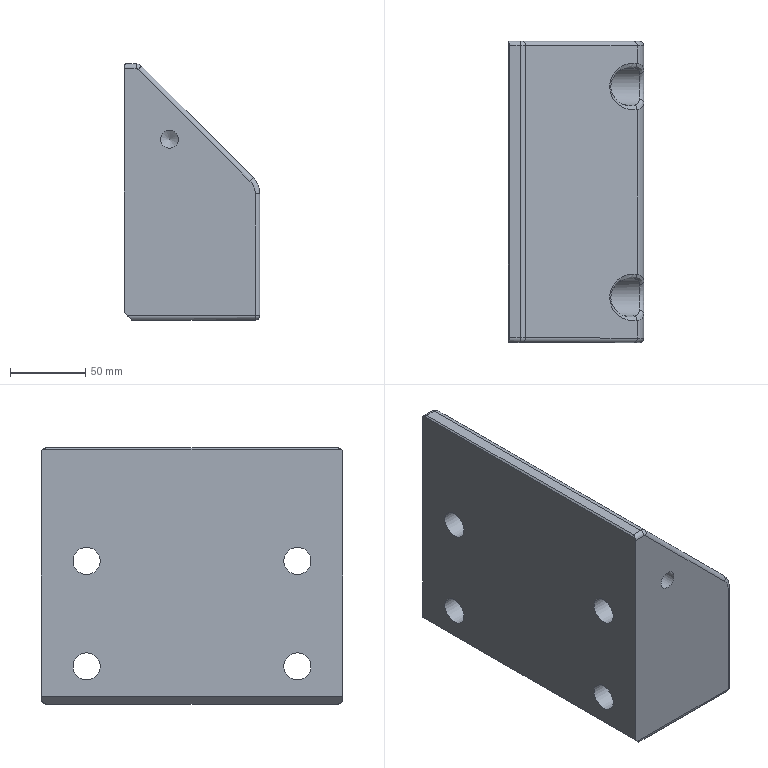Part | NX | features solid 2 | 1 solid | 54 faces | box 90 x 200 x 170 mm | volume 2273668 mm3 | cylinder 23 | plane 13 | torus 8 | spline 6 | cone 2 | sphere 2 | commonest cylinder face diameters 6 x9 18 x4 25 x4 30 x3 12 x2 10 x1